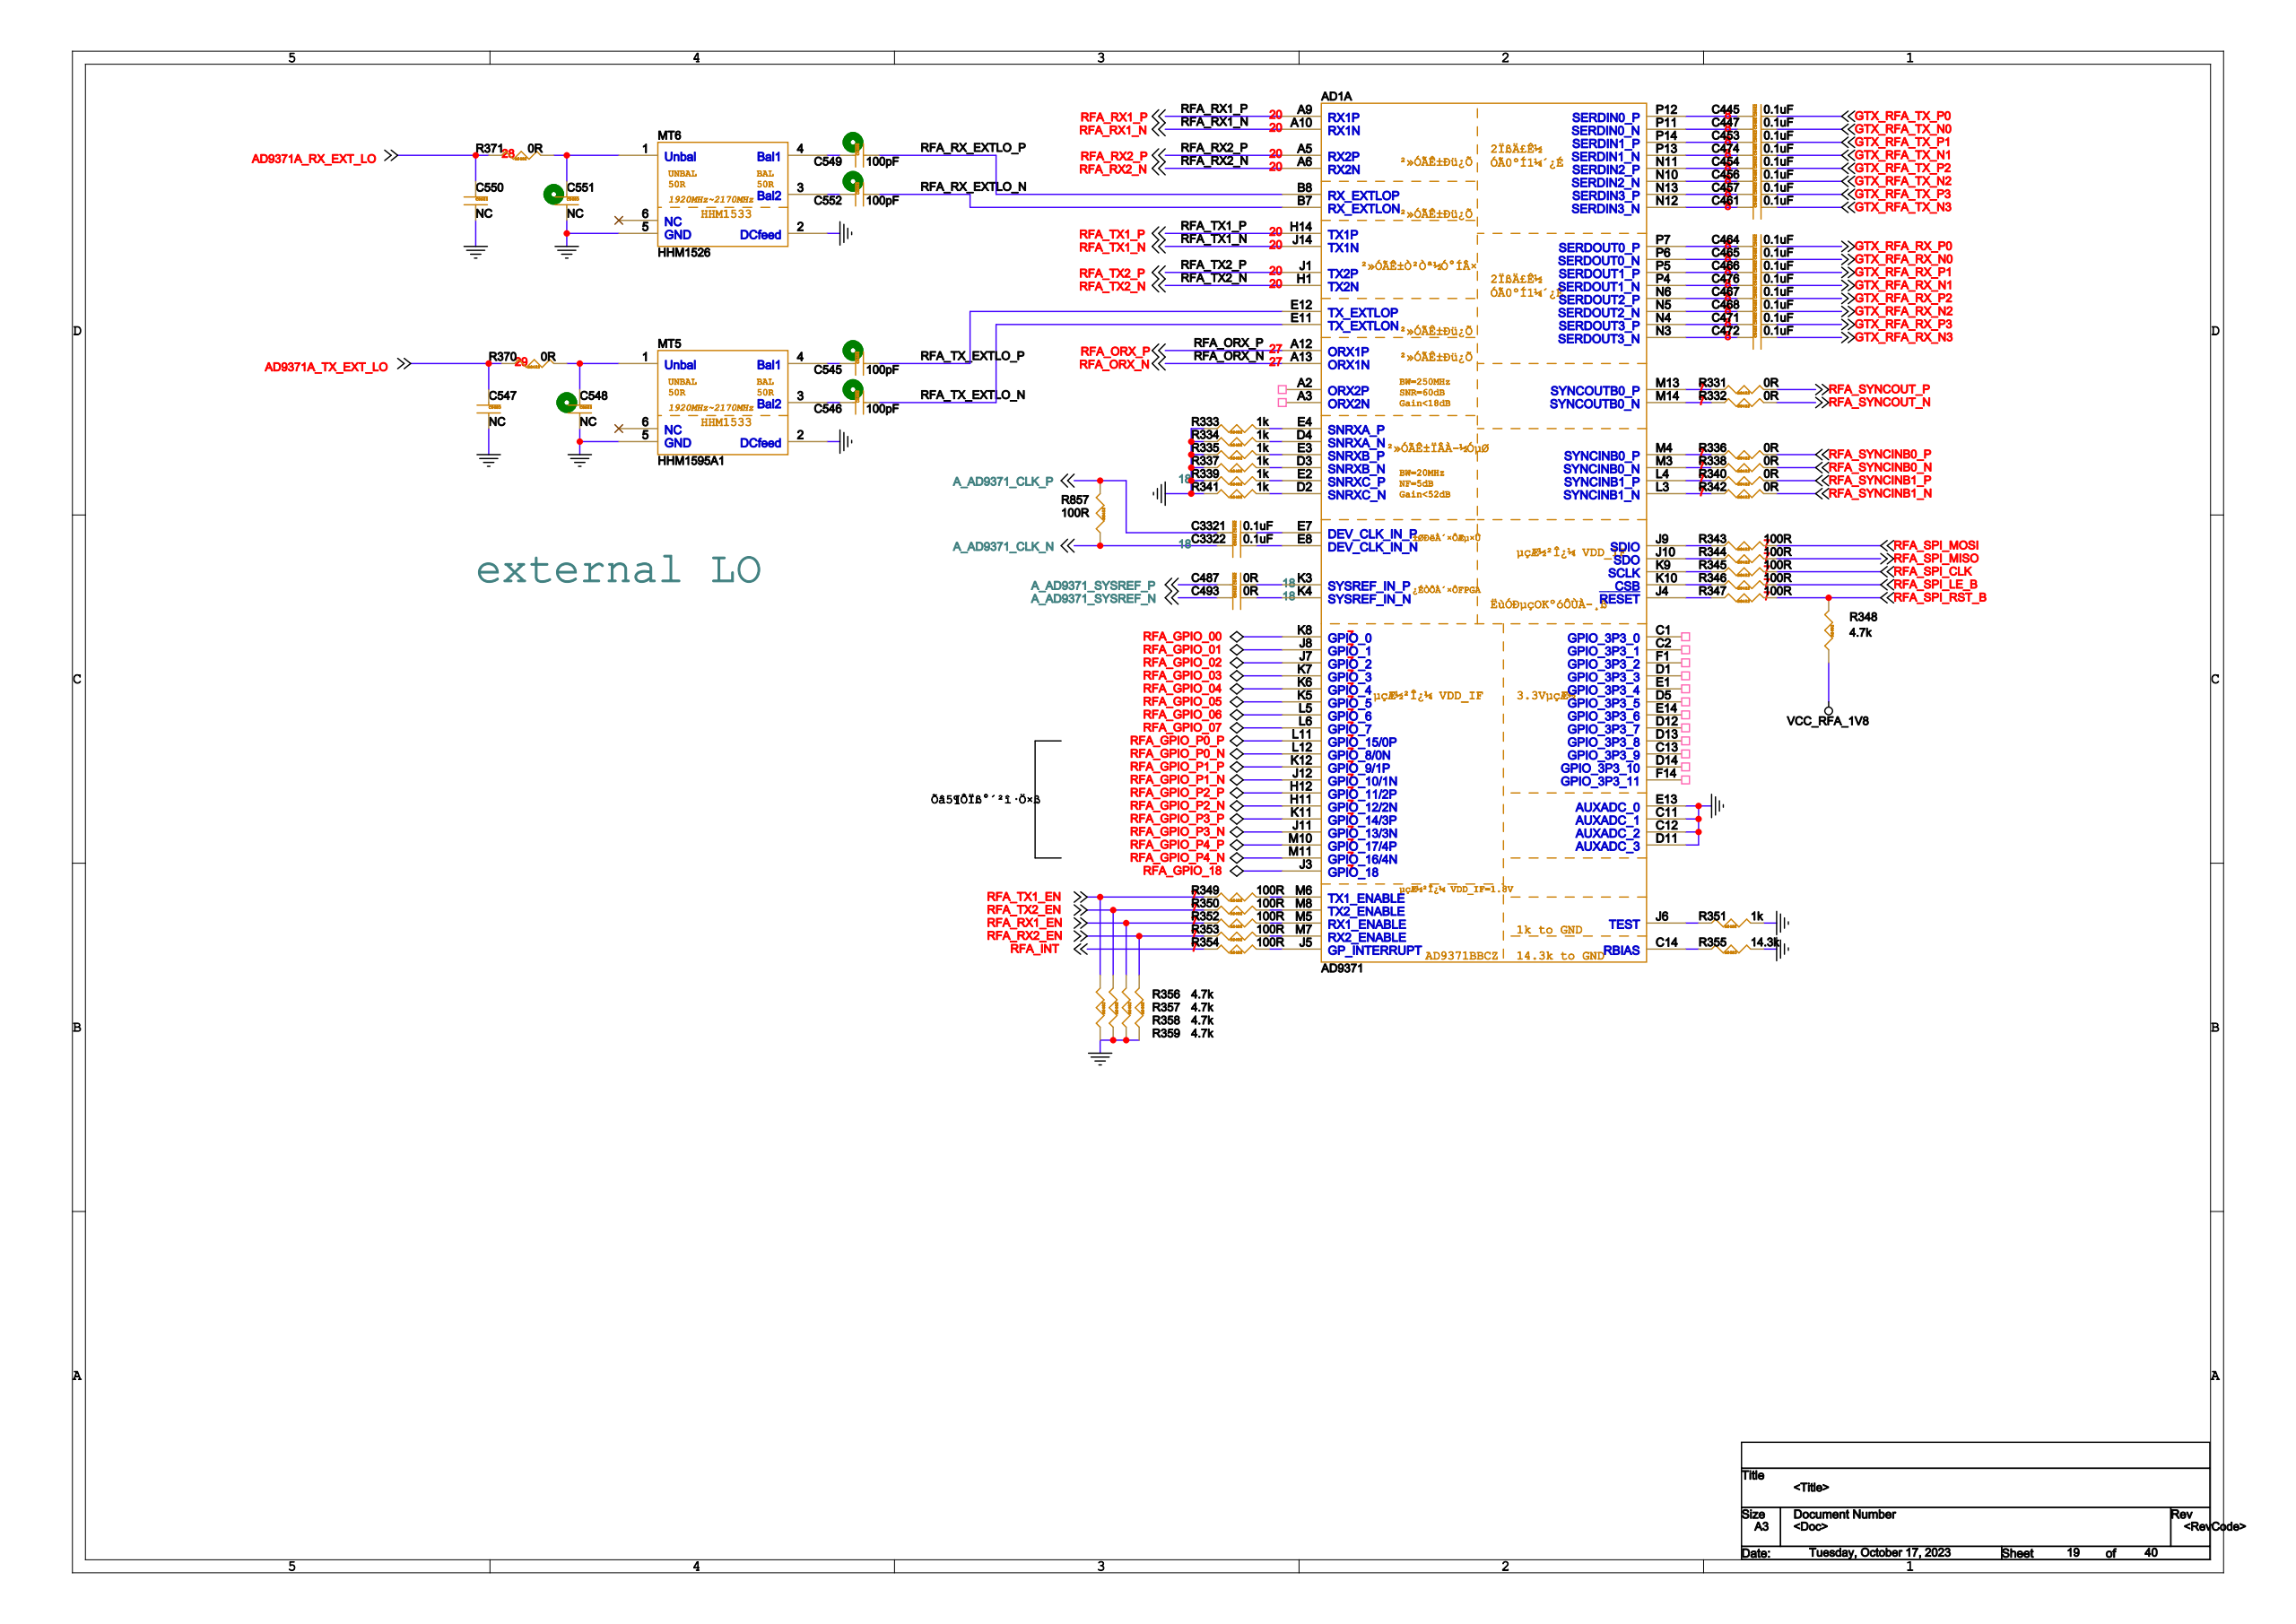Circuit board | Cadence Allegro | 1793 parts | 1223 nets | one sheet of the schematic
Parts on this sheet (reference | value | footprint):
AD1 | AD9371 | BGA196
C445 | 0.1uF | C0402
C447 | 0.1uF | C0402
C453 | 0.1uF | C0402
C454 | 0.1uF | C0402
C456 | 0.1uF | C0402
C457 | 0.1uF | C0402
C461 | 0.1uF | C0402
C464 | 0.1uF | C0402
C465 | 0.1uF | C0402
C466 | 0.1uF | C0402
C467 | 0.1uF | C0402
C468 | 0.1uF | C0402
C471 | 0.1uF | C0402
C472 | 0.1uF | C0402
C474 | 0.1uF | C0402
C476 | 0.1uF | C0402
C487 | 0R | C0402
C493 | 0R | C0402
C545 | 100pF | C0402
C546 | 100pF | C0402
C547 | NC | C0402
C548 | NC | C0402
C549 | 100pF | C0402
C550 | NC | C0402
C551 | NC | C0402
C552 | 100pF | C0402
C3321 | 0.1uF | C0402
C3322 | 0.1uF | C0402
MT5 | HHM1595A1 | HHM1595A1
MT6 | HHM1526 | HHM1595A1
R331 | 0R | R0402
R332 | 0R | R0402
R333 | 1k | R0402
R334 | 1k | R0402
R335 | 1k | R0402
R336 | 0R | R0402
R337 | 1k | R0402
R338 | 0R | R0402
R339 | 1k | R0402
R340 | 0R | R0402
R341 | 1k | R0402
R342 | 0R | R0402
R343 | 100R | R0402
R344 | 100R | R0402
R345 | 100R | R0402
R346 | 100R | R0402
R347 | 100R | R0402
R348 | 4.7k | R0402
R349 | 100R | R0402
R350 | 100R | R0402
R351 | 1k | R0402
R352 | 100R | R0402
R353 | 100R | R0402
R354 | 100R | R0402
R355 | 14.3k | R0402
R356 | 4.7k | R0402
R357 | 4.7k | R0402
R358 | 4.7k | R0402
R359 | 4.7k | R0402
R370 | 0R | R0402
R371 | 0R | R0402
R857 | 100R | R0402
Nets of these parts (net: part-pin ...):
GND: C547-2 C548-2 C550-2 C551-2 MT5-2 MT5-5 MT6-2 MT6-5 R333-1 R334-1 R335-1 R337-1 R339-1 R341-1 R351-2 R355-2 R356-1 R357-1 R358-1 R359-1 AD1-C11 AD1-C12 AD1-D11 AD1-E13
N716439: C549-1 MT6-4
N716521: C552-1 MT6-3
N716427: C551-1 MT6-1 R371-2
VCC_RFA_1V8: R348-1
AD9371A_TX_EXT_LO: C547-1 R370-1
N716157: C548-1 MT5-1 R370-2
AD9371A_RX_EXT_LO: C550-1 R371-1
N1530063: R346-1 AD1-K10
N16890952: C3322-2 AD1-E8
N16890949: C3321-2 AD1-E7
RFA_GPIO_00: AD1-K8
RFA_GPIO_01: AD1-J8
RFA_GPIO_P1_N: AD1-J12
RFA_GPIO_P2_P: AD1-H12
RFA_GPIO_P2_N: AD1-H11
RFA_GPIO_P3_N: AD1-J11
RFA_GPIO_P3_P: AD1-K11
RFA_GPIO_P0_P: AD1-L11
RFA_GPIO_P4_N: AD1-M11
RFA_GPIO_P4_P: AD1-M10
RFA_GPIO_18: AD1-J3
RFA_GPIO_02: AD1-J7
RFA_GPIO_03: AD1-K7
RFA_GPIO_04: AD1-K6
RFA_GPIO_05: AD1-K5
RFA_GPIO_06: AD1-L5
RFA_GPIO_07: AD1-L6
RFA_GPIO_P0_N: AD1-L12
RFA_GPIO_P1_P: AD1-K12
N18256569: R354-2 AD1-J5
RFA_ORX_N: AD1-A13
RFA_ORX_P: AD1-A12
N713623: R355-1 AD1-C14
RFA_RX1_N: AD1-A10
RFA_RX1_P: AD1-A9
N18256571: R352-2 AD1-M5
RFA_RX2_N: AD1-A6
RFA_RX2_P: AD1-A5
N18256568: R353-2 AD1-M7
RFA_RX_EXTLO_N: C552-2 AD1-B7
RFA_RX_EXTLO_P: C549-2 AD1-B8
N1530067: R347-1 AD1-J4
N1530053: R345-1 AD1-K9
N1529915: R343-1 AD1-J9
N1530049: R344-1 AD1-J10
N708845: C447-1 AD1-P11
N708693: C445-1 AD1-P12
N708999: C474-1 AD1-P13
N708911: C453-1 AD1-P14
N709161: C456-1 AD1-N10
N709091: C454-1 AD1-N11
N709385: C461-1 AD1-N12
N709281: C457-1 AD1-N13
N1538607: C465-1 AD1-P6
N1538603: C464-1 AD1-P7
N1538615: C476-1 AD1-P4
N1538611: C466-1 AD1-P5
N1538629: C468-1 AD1-N5
N1538619: C467-1 AD1-N6
N1538637: C472-1 AD1-N3
N1538633: C471-1 AD1-N4
N710529: R334-2 AD1-D4
N710465: R333-2 AD1-E4
N710693: R337-2 AD1-D3
N710599: R335-2 AD1-E3
N710905: R341-2 AD1-D2
N710803: R339-2 AD1-E2
N18257151: R338-1 AD1-M3
N18257146: R336-1 AD1-M4
N18257150: R342-1 AD1-L3
N18257149: R340-1 AD1-L4
N18257147: R332-1 AD1-M14
N18257148: R331-1 AD1-M13
N711499: C493-2 AD1-K4
N711453: C487-2 AD1-K3
N713417: R351-1 AD1-J6
RFA_TX1_N: AD1-J14
RFA_TX1_P: AD1-H14
N18256570: R349-2 AD1-M6
RFA_TX2_N: AD1-H1
RFA_TX2_P: AD1-J1
N18256572: R350-2 AD1-M8
RFA_TX_EXTLO_N: C546-2 AD1-E11
RFA_TX_EXTLO_P: C545-2 AD1-E12
A_AD9371_CLK_P: C3321-1 R857-2
A_AD9371_CLK_N: C3322-1 R857-1
GTX_RFA_TX_P0: C445-2
GTX_RFA_TX_N0: C447-2
GTX_RFA_TX_P1: C453-2
GTX_RFA_TX_P2: C454-2
GTX_RFA_TX_N2: C456-2
GTX_RFA_TX_P3: C457-2
GTX_RFA_TX_N3: C461-2
GTX_RFA_RX_P0: C464-2
GTX_RFA_RX_N0: C465-2
GTX_RFA_RX_P1: C466-2
GTX_RFA_RX_P2: C467-2
GTX_RFA_RX_N2: C468-2
GTX_RFA_RX_P3: C471-2
GTX_RFA_RX_N3: C472-2
GTX_RFA_TX_N1: C474-2
GTX_RFA_RX_N1: C476-2
A_AD9371_SYSREF_P: C487-1
A_AD9371_SYSREF_N: C493-1
N716169: C545-1 MT5-4
N716267: C546-1 MT5-3
RFA_SYNCOUT_P: R331-2
RFA_SYNCOUT_N: R332-2
RFA_SYNCINB0_P: R336-2
RFA_SYNCINB0_N: R338-2
RFA_SYNCINB1_P: R340-2
RFA_SYNCINB1_N: R342-2
RFA_SPI_MOSI: R343-2
RFA_SPI_MISO: R344-2
RFA_SPI_CLK: R345-2
RFA_SPI_LE_B: R346-2
RFA_SPI_RST_B: R347-2 R348-2
RFA_TX1_EN: R349-1 R356-2
RFA_TX2_EN: R350-1 R357-2
RFA_RX1_EN: R352-1 R358-2
RFA_RX2_EN: R353-1 R359-2
RFA_INT: R354-1